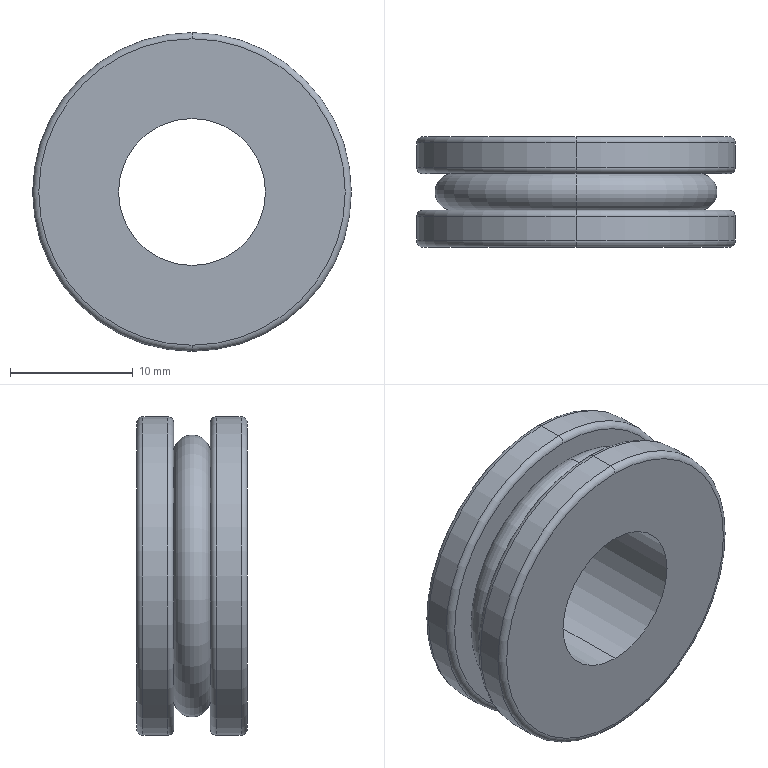Part | SolidWorks | features Fillet 1, Revolution 1 | 1 solid | 20 faces | box 26 x 9 x 26 mm | volume 3329 mm3 | torus 10 | cylinder 6 | plane 4 | commonest cylinder face diameters 26 x4 12 x2
STEP:
#1=CARTESIAN_POINT('',(0.,-3.,-12.5));
#2=VERTEX_POINT('',#1);
#3=CARTESIAN_POINT('',(0.,-3.,12.5));
#4=VERTEX_POINT('',#3);
#5=CARTESIAN_POINT('',(0.,-3.,0.));
#6=DIRECTION('',(0.,-1.,0.));
#7=DIRECTION('',(0.,0.,1.));
#8=AXIS2_PLACEMENT_3D('',#5,#6,#7);
#9=CIRCLE('',#8,12.5);
#10=EDGE_CURVE('',#2,#4,#9,.T.);
#11=ORIENTED_EDGE('',*,*,#10,.F.);
#12=CARTESIAN_POINT('',(0.,-2.5,-13.));
#13=VERTEX_POINT('',#12);
#14=CARTESIAN_POINT('',(0.,-2.5,-12.5));
#15=DIRECTION('',(1.,0.,0.));
#16=DIRECTION('',(0.,0.,-1.));
#17=AXIS2_PLACEMENT_3D('',#14,#15,#16);
#18=CIRCLE('',#17,0.5);
#19=EDGE_CURVE('',#2,#13,#18,.T.);
#20=ORIENTED_EDGE('',*,*,#19,.T.);
#21=CARTESIAN_POINT('',(0.,-2.5,13.));
#22=VERTEX_POINT('',#21);
#23=CARTESIAN_POINT('',(0.,-2.5,0.));
#24=DIRECTION('',(0.,1.,0.));
#25=DIRECTION('',(0.,0.,1.));
#26=AXIS2_PLACEMENT_3D('',#23,#24,#25);
#27=CIRCLE('',#26,13.);
#28=EDGE_CURVE('',#22,#13,#27,.T.);
#29=ORIENTED_EDGE('',*,*,#28,.F.);
#30=CARTESIAN_POINT('',(0.,-2.5,12.5));
#31=DIRECTION('',(-1.,0.,0.));
#32=DIRECTION('',(0.,0.,1.));
#33=AXIS2_PLACEMENT_3D('',#30,#31,#32);
#34=CIRCLE('',#33,0.5);
#35=EDGE_CURVE('',#4,#22,#34,.T.);
#36=ORIENTED_EDGE('',*,*,#35,.F.);
#37=EDGE_LOOP('',(#11,#20,#29,#36));
#38=FACE_OUTER_BOUND('',#37,.T.);
#39=CARTESIAN_POINT('',(0.,-2.5,0.));
#40=DIRECTION('',(0.,1.,0.));
#41=DIRECTION('',(0.,0.,1.));
#42=AXIS2_PLACEMENT_3D('',#39,#40,#41);
#43=TOROIDAL_SURFACE('',#42,12.5,0.5);
#44=ADVANCED_FACE('',(#38),#43,.T.);
#45=CARTESIAN_POINT('',(0.,0.,12.5));
#46=VERTEX_POINT('',#45);
#47=CARTESIAN_POINT('',(0.,0.,-12.5));
#48=VERTEX_POINT('',#47);
#49=CARTESIAN_POINT('',(0.,0.,0.));
#50=DIRECTION('',(0.,1.,0.));
#51=DIRECTION('',(0.,0.,-1.));
#52=AXIS2_PLACEMENT_3D('',#49,#50,#51);
#53=CIRCLE('',#52,12.5);
#54=EDGE_CURVE('',#46,#48,#53,.T.);
#55=ORIENTED_EDGE('',*,*,#54,.F.);
#56=CARTESIAN_POINT('',(0.,-0.5,13.));
#57=VERTEX_POINT('',#56);
#58=CARTESIAN_POINT('',(0.,-0.5,12.5));
#59=DIRECTION('',(1.,0.,0.));
#60=DIRECTION('',(0.,0.,-1.));
#61=AXIS2_PLACEMENT_3D('',#58,#59,#60);
#62=CIRCLE('',#61,0.5);
#63=EDGE_CURVE('',#46,#57,#62,.T.);
#64=ORIENTED_EDGE('',*,*,#63,.T.);
#65=CARTESIAN_POINT('',(0.,-0.5,-13.));
#66=VERTEX_POINT('',#65);
#67=CARTESIAN_POINT('',(0.,-0.5,0.));
#68=DIRECTION('',(0.,-1.,0.));
#69=DIRECTION('',(0.,0.,-1.));
#70=AXIS2_PLACEMENT_3D('',#67,#68,#69);
#71=CIRCLE('',#70,13.);
#72=EDGE_CURVE('',#66,#57,#71,.T.);
#73=ORIENTED_EDGE('',*,*,#72,.F.);
#74=CARTESIAN_POINT('',(0.,-0.5,-12.5));
#75=DIRECTION('',(-1.,0.,0.));
#76=DIRECTION('',(0.,0.,1.));
#77=AXIS2_PLACEMENT_3D('',#74,#75,#76);
#78=CIRCLE('',#77,0.5);
#79=EDGE_CURVE('',#48,#66,#78,.T.);
#80=ORIENTED_EDGE('',*,*,#79,.F.);
#81=EDGE_LOOP('',(#55,#64,#73,#80));
#82=FACE_OUTER_BOUND('',#81,.T.);
#83=CARTESIAN_POINT('',(0.,-0.5,0.));
#84=DIRECTION('',(0.,-1.,0.));
#85=DIRECTION('',(0.,0.,-1.));
#86=AXIS2_PLACEMENT_3D('',#83,#84,#85);
#87=TOROIDAL_SURFACE('',#86,12.5,0.5);
#88=ADVANCED_FACE('',(#82),#87,.T.);
#89=CARTESIAN_POINT('',(0.,-6.,12.5));
#90=VERTEX_POINT('',#89);
#91=CARTESIAN_POINT('',(0.,-6.,-12.5));
#92=VERTEX_POINT('',#91);
#93=CARTESIAN_POINT('',(0.,-6.,0.));
#94=DIRECTION('',(0.,1.,0.));
#95=DIRECTION('',(0.,0.,-1.));
#96=AXIS2_PLACEMENT_3D('',#93,#94,#95);
#97=CIRCLE('',#96,12.5);
#98=EDGE_CURVE('',#90,#92,#97,.T.);
#99=ORIENTED_EDGE('',*,*,#98,.F.);
#100=CARTESIAN_POINT('',(0.,-6.5,13.));
#101=VERTEX_POINT('',#100);
#102=CARTESIAN_POINT('',(0.,-6.5,12.5));
#103=DIRECTION('',(1.,0.,0.));
#104=DIRECTION('',(0.,0.,-1.));
#105=AXIS2_PLACEMENT_3D('',#102,#103,#104);
#106=CIRCLE('',#105,0.5);
#107=EDGE_CURVE('',#90,#101,#106,.T.);
#108=ORIENTED_EDGE('',*,*,#107,.T.);
#109=CARTESIAN_POINT('',(0.,-6.5,-13.));
#110=VERTEX_POINT('',#109);
#111=CARTESIAN_POINT('',(0.,-6.5,0.));
#112=DIRECTION('',(0.,-1.,0.));
#113=DIRECTION('',(0.,0.,-1.));
#114=AXIS2_PLACEMENT_3D('',#111,#112,#113);
#115=CIRCLE('',#114,13.);
#116=EDGE_CURVE('',#110,#101,#115,.T.);
#117=ORIENTED_EDGE('',*,*,#116,.F.);
#118=CARTESIAN_POINT('',(0.,-6.5,-12.5));
#119=DIRECTION('',(-1.,0.,0.));
#120=DIRECTION('',(0.,0.,1.));
#121=AXIS2_PLACEMENT_3D('',#118,#119,#120);
#122=CIRCLE('',#121,0.5);
#123=EDGE_CURVE('',#92,#110,#122,.T.);
#124=ORIENTED_EDGE('',*,*,#123,.F.);
#125=EDGE_LOOP('',(#99,#108,#117,#124));
#126=FACE_OUTER_BOUND('',#125,.T.);
#127=CARTESIAN_POINT('',(0.,-6.5,0.));
#128=DIRECTION('',(0.,-1.,0.));
#129=DIRECTION('',(0.,0.,-1.));
#130=AXIS2_PLACEMENT_3D('',#127,#128,#129);
#131=TOROIDAL_SURFACE('',#130,12.5,0.5);
#132=ADVANCED_FACE('',(#126),#131,.T.);
#133=CARTESIAN_POINT('',(0.,-9.,-12.5));
#134=VERTEX_POINT('',#133);
#135=CARTESIAN_POINT('',(0.,-9.,12.5));
#136=VERTEX_POINT('',#135);
#137=CARTESIAN_POINT('',(0.,-9.,0.));
#138=DIRECTION('',(0.,-1.,0.));
#139=DIRECTION('',(0.,0.,1.));
#140=AXIS2_PLACEMENT_3D('',#137,#138,#139);
#141=CIRCLE('',#140,12.5);
#142=EDGE_CURVE('',#134,#136,#141,.T.);
#143=ORIENTED_EDGE('',*,*,#142,.F.);
#144=CARTESIAN_POINT('',(0.,-8.5,-13.));
#145=VERTEX_POINT('',#144);
#146=CARTESIAN_POINT('',(0.,-8.5,-12.5));
#147=DIRECTION('',(1.,0.,0.));
#148=DIRECTION('',(0.,0.,-1.));
#149=AXIS2_PLACEMENT_3D('',#146,#147,#148);
#150=CIRCLE('',#149,0.5);
#151=EDGE_CURVE('',#134,#145,#150,.T.);
#152=ORIENTED_EDGE('',*,*,#151,.T.);
#153=CARTESIAN_POINT('',(0.,-8.5,13.));
#154=VERTEX_POINT('',#153);
#155=CARTESIAN_POINT('',(0.,-8.5,0.));
#156=DIRECTION('',(0.,1.,0.));
#157=DIRECTION('',(0.,0.,1.));
#158=AXIS2_PLACEMENT_3D('',#155,#156,#157);
#159=CIRCLE('',#158,13.);
#160=EDGE_CURVE('',#154,#145,#159,.T.);
#161=ORIENTED_EDGE('',*,*,#160,.F.);
#162=CARTESIAN_POINT('',(0.,-8.5,12.5));
#163=DIRECTION('',(-1.,0.,0.));
#164=DIRECTION('',(0.,0.,1.));
#165=AXIS2_PLACEMENT_3D('',#162,#163,#164);
#166=CIRCLE('',#165,0.5);
#167=EDGE_CURVE('',#136,#154,#166,.T.);
#168=ORIENTED_EDGE('',*,*,#167,.F.);
#169=EDGE_LOOP('',(#143,#152,#161,#168));
#170=FACE_OUTER_BOUND('',#169,.T.);
#171=CARTESIAN_POINT('',(0.,-8.5,0.));
#172=DIRECTION('',(0.,1.,0.));
#173=DIRECTION('',(0.,0.,1.));
#174=AXIS2_PLACEMENT_3D('',#171,#172,#173);
#175=TOROIDAL_SURFACE('',#174,12.5,0.5);
#176=ADVANCED_FACE('',(#170),#175,.T.);
#177=CARTESIAN_POINT('',(0.,-9.,-6.));
#178=VERTEX_POINT('',#177);
#179=CARTESIAN_POINT('',(0.,-9.,6.));
#180=VERTEX_POINT('',#179);
#181=CARTESIAN_POINT('',(0.,-9.,0.));
#182=DIRECTION('',(0.,1.,0.));
#183=DIRECTION('',(0.,0.,1.));
#184=AXIS2_PLACEMENT_3D('',#181,#182,#183);
#185=CIRCLE('',#184,6.);
#186=EDGE_CURVE('',#178,#180,#185,.T.);
#187=ORIENTED_EDGE('',*,*,#186,.F.);
#188=CARTESIAN_POINT('',(0.,0.,-6.));
#189=VERTEX_POINT('',#188);
#190=CARTESIAN_POINT('',(0.,0.,-6.));
#191=DIRECTION('',(0.,1.,0.));
#192=VECTOR('',#191,1000.);
#193=LINE('',#190,#192);
#194=EDGE_CURVE('',#178,#189,#193,.T.);
#195=ORIENTED_EDGE('',*,*,#194,.T.);
#196=CARTESIAN_POINT('',(0.,0.,6.));
#197=VERTEX_POINT('',#196);
#198=CARTESIAN_POINT('',(0.,0.,0.));
#199=DIRECTION('',(0.,1.,0.));
#200=DIRECTION('',(0.,0.,1.));
#201=AXIS2_PLACEMENT_3D('',#198,#199,#200);
#202=CIRCLE('',#201,6.);
#203=EDGE_CURVE('',#189,#197,#202,.T.);
#204=ORIENTED_EDGE('',*,*,#203,.T.);
#205=CARTESIAN_POINT('',(0.,0.,6.));
#206=DIRECTION('',(0.,1.,0.));
#207=VECTOR('',#206,1000.);
#208=LINE('',#205,#207);
#209=EDGE_CURVE('',#180,#197,#208,.T.);
#210=ORIENTED_EDGE('',*,*,#209,.F.);
#211=EDGE_LOOP('',(#187,#195,#204,#210));
#212=FACE_OUTER_BOUND('',#211,.T.);
#213=CARTESIAN_POINT('',(0.,0.,0.));
#214=DIRECTION('',(0.,1.,0.));
#215=DIRECTION('',(0.,0.,1.));
#216=AXIS2_PLACEMENT_3D('',#213,#214,#215);
#217=CYLINDRICAL_SURFACE('',#216,6.);
#218=ADVANCED_FACE('',(#212),#217,.F.);
#219=ORIENTED_EDGE('',*,*,#160,.T.);
#220=CARTESIAN_POINT('',(0.,0.,-13.));
#221=DIRECTION('',(0.,1.,0.));
#222=VECTOR('',#221,1000.);
#223=LINE('',#220,#222);
#224=EDGE_CURVE('',#145,#110,#223,.T.);
#225=ORIENTED_EDGE('',*,*,#224,.T.);
#226=ORIENTED_EDGE('',*,*,#116,.T.);
#227=CARTESIAN_POINT('',(0.,0.,13.));
#228=DIRECTION('',(0.,1.,0.));
#229=VECTOR('',#228,1000.);
#230=LINE('',#227,#229);
#231=EDGE_CURVE('',#154,#101,#230,.T.);
#232=ORIENTED_EDGE('',*,*,#231,.F.);
#233=EDGE_LOOP('',(#219,#225,#226,#232));
#234=FACE_OUTER_BOUND('',#233,.T.);
#235=CARTESIAN_POINT('',(0.,0.,0.));
#236=DIRECTION('',(0.,1.,0.));
#237=DIRECTION('',(0.,0.,1.));
#238=AXIS2_PLACEMENT_3D('',#235,#236,#237);
#239=CYLINDRICAL_SURFACE('',#238,13.);
#240=ADVANCED_FACE('',(#234),#239,.T.);
#241=CARTESIAN_POINT('',(0.,-6.,10.));
#242=VERTEX_POINT('',#241);
#243=CARTESIAN_POINT('',(0.,-6.,-10.));
#244=VERTEX_POINT('',#243);
#245=CARTESIAN_POINT('',(0.,-6.,0.));
#246=DIRECTION('',(0.,1.,0.));
#247=DIRECTION('',(0.,0.,1.));
#248=AXIS2_PLACEMENT_3D('',#245,#246,#247);
#249=CIRCLE('',#248,10.);
#250=EDGE_CURVE('',#242,#244,#249,.T.);
#251=ORIENTED_EDGE('',*,*,#250,.T.);
#252=CARTESIAN_POINT('',(0.,-3.,-10.));
#253=VERTEX_POINT('',#252);
#254=CARTESIAN_POINT('',(0.,-4.5,-10.));
#255=DIRECTION('',(1.,0.,0.));
#256=DIRECTION('',(0.,0.,-1.));
#257=AXIS2_PLACEMENT_3D('',#254,#255,#256);
#258=CIRCLE('',#257,1.5);
#259=EDGE_CURVE('',#244,#253,#258,.T.);
#260=ORIENTED_EDGE('',*,*,#259,.T.);
#261=CARTESIAN_POINT('',(0.,-3.,10.));
#262=VERTEX_POINT('',#261);
#263=CARTESIAN_POINT('',(0.,-3.,0.));
#264=DIRECTION('',(0.,1.,0.));
#265=DIRECTION('',(0.,0.,1.));
#266=AXIS2_PLACEMENT_3D('',#263,#264,#265);
#267=CIRCLE('',#266,10.);
#268=EDGE_CURVE('',#262,#253,#267,.T.);
#269=ORIENTED_EDGE('',*,*,#268,.F.);
#270=CARTESIAN_POINT('',(0.,-4.5,10.));
#271=DIRECTION('',(-1.,0.,0.));
#272=DIRECTION('',(0.,0.,1.));
#273=AXIS2_PLACEMENT_3D('',#270,#271,#272);
#274=CIRCLE('',#273,1.5);
#275=EDGE_CURVE('',#242,#262,#274,.T.);
#276=ORIENTED_EDGE('',*,*,#275,.F.);
#277=EDGE_LOOP('',(#251,#260,#269,#276));
#278=FACE_OUTER_BOUND('',#277,.T.);
#279=CARTESIAN_POINT('',(0.,-4.5,0.));
#280=DIRECTION('',(0.,1.,0.));
#281=DIRECTION('',(0.,0.,1.));
#282=AXIS2_PLACEMENT_3D('',#279,#280,#281);
#283=TOROIDAL_SURFACE('',#282,10.,1.5);
#284=ADVANCED_FACE('',(#278),#283,.T.);
#285=ORIENTED_EDGE('',*,*,#28,.T.);
#286=CARTESIAN_POINT('',(0.,0.,-13.));
#287=DIRECTION('',(0.,1.,0.));
#288=VECTOR('',#287,1000.);
#289=LINE('',#286,#288);
#290=EDGE_CURVE('',#13,#66,#289,.T.);
#291=ORIENTED_EDGE('',*,*,#290,.T.);
#292=ORIENTED_EDGE('',*,*,#72,.T.);
#293=CARTESIAN_POINT('',(0.,0.,13.));
#294=DIRECTION('',(0.,1.,0.));
#295=VECTOR('',#294,1000.);
#296=LINE('',#293,#295);
#297=EDGE_CURVE('',#22,#57,#296,.T.);
#298=ORIENTED_EDGE('',*,*,#297,.F.);
#299=EDGE_LOOP('',(#285,#291,#292,#298));
#300=FACE_OUTER_BOUND('',#299,.T.);
#301=CARTESIAN_POINT('',(0.,0.,0.));
#302=DIRECTION('',(0.,1.,0.));
#303=DIRECTION('',(0.,0.,1.));
#304=AXIS2_PLACEMENT_3D('',#301,#302,#303);
#305=CYLINDRICAL_SURFACE('',#304,13.);
#306=ADVANCED_FACE('',(#300),#305,.T.);
#307=ORIENTED_EDGE('',*,*,#290,.F.);
#308=CARTESIAN_POINT('',(0.,-2.5,0.));
#309=DIRECTION('',(0.,1.,0.));
#310=DIRECTION('',(0.,0.,1.));
#311=AXIS2_PLACEMENT_3D('',#308,#309,#310);
#312=CIRCLE('',#311,13.);
#313=EDGE_CURVE('',#13,#22,#312,.T.);
#314=ORIENTED_EDGE('',*,*,#313,.T.);
#315=ORIENTED_EDGE('',*,*,#297,.T.);
#316=CARTESIAN_POINT('',(0.,-0.5,0.));
#317=DIRECTION('',(0.,-1.,0.));
#318=DIRECTION('',(0.,0.,-1.));
#319=AXIS2_PLACEMENT_3D('',#316,#317,#318);
#320=CIRCLE('',#319,13.);
#321=EDGE_CURVE('',#57,#66,#320,.T.);
#322=ORIENTED_EDGE('',*,*,#321,.T.);
#323=EDGE_LOOP('',(#307,#314,#315,#322));
#324=FACE_OUTER_BOUND('',#323,.T.);
#325=CARTESIAN_POINT('',(0.,0.,0.));
#326=DIRECTION('',(0.,1.,0.));
#327=DIRECTION('',(0.,0.,1.));
#328=AXIS2_PLACEMENT_3D('',#325,#326,#327);
#329=CYLINDRICAL_SURFACE('',#328,13.);
#330=ADVANCED_FACE('',(#324),#329,.T.);
#331=CARTESIAN_POINT('',(0.,-3.,0.));
#332=DIRECTION('',(0.,-1.,0.));
#333=DIRECTION('',(0.,0.,1.));
#334=AXIS2_PLACEMENT_3D('',#331,#332,#333);
#335=CIRCLE('',#334,12.5);
#336=EDGE_CURVE('',#4,#2,#335,.T.);
#337=ORIENTED_EDGE('',*,*,#336,.T.);
#338=ORIENTED_EDGE('',*,*,#10,.T.);
#339=EDGE_LOOP('',(#337,#338));
#340=FACE_OUTER_BOUND('',#339,.T.);
#341=ORIENTED_EDGE('',*,*,#268,.T.);
#342=CARTESIAN_POINT('',(0.,-3.,0.));
#343=DIRECTION('',(0.,1.,0.));
#344=DIRECTION('',(0.,0.,1.));
#345=AXIS2_PLACEMENT_3D('',#342,#343,#344);
#346=CIRCLE('',#345,10.);
#347=EDGE_CURVE('',#253,#262,#346,.T.);
#348=ORIENTED_EDGE('',*,*,#347,.T.);
#349=EDGE_LOOP('',(#341,#348));
#350=FACE_BOUND('',#349,.T.);
#351=CARTESIAN_POINT('',(13.,-3.,0.));
#352=DIRECTION('',(0.,1.,0.));
#353=DIRECTION('',(0.,0.,1.));
#354=AXIS2_PLACEMENT_3D('',#351,#352,#353);
#355=PLANE('',#354);
#356=ADVANCED_FACE('',(#340,#350),#355,.F.);
#357=ORIENTED_EDGE('',*,*,#259,.F.);
#358=CARTESIAN_POINT('',(0.,-6.,0.));
#359=DIRECTION('',(0.,1.,0.));
#360=DIRECTION('',(0.,0.,1.));
#361=AXIS2_PLACEMENT_3D('',#358,#359,#360);
#362=CIRCLE('',#361,10.);
#363=EDGE_CURVE('',#244,#242,#362,.T.);
#364=ORIENTED_EDGE('',*,*,#363,.T.);
#365=ORIENTED_EDGE('',*,*,#275,.T.);
#366=ORIENTED_EDGE('',*,*,#347,.F.);
#367=EDGE_LOOP('',(#357,#364,#365,#366));
#368=FACE_OUTER_BOUND('',#367,.T.);
#369=CARTESIAN_POINT('',(0.,-4.5,0.));
#370=DIRECTION('',(0.,1.,0.));
#371=DIRECTION('',(0.,0.,1.));
#372=AXIS2_PLACEMENT_3D('',#369,#370,#371);
#373=TOROIDAL_SURFACE('',#372,10.,1.5);
#374=ADVANCED_FACE('',(#368),#373,.T.);
#375=CARTESIAN_POINT('',(0.,-6.,0.));
#376=DIRECTION('',(0.,1.,0.));
#377=DIRECTION('',(0.,0.,-1.));
#378=AXIS2_PLACEMENT_3D('',#375,#376,#377);
#379=CIRCLE('',#378,12.5);
#380=EDGE_CURVE('',#92,#90,#379,.T.);
#381=ORIENTED_EDGE('',*,*,#380,.T.);
#382=ORIENTED_EDGE('',*,*,#98,.T.);
#383=EDGE_LOOP('',(#381,#382));
#384=FACE_OUTER_BOUND('',#383,.T.);
#385=ORIENTED_EDGE('',*,*,#250,.F.);
#386=ORIENTED_EDGE('',*,*,#363,.F.);
#387=EDGE_LOOP('',(#385,#386));
#388=FACE_BOUND('',#387,.T.);
#389=CARTESIAN_POINT('',(10.,-6.,0.));
#390=DIRECTION('',(0.,-1.,0.));
#391=DIRECTION('',(0.,0.,-1.));
#392=AXIS2_PLACEMENT_3D('',#389,#390,#391);
#393=PLANE('',#392);
#394=ADVANCED_FACE('',(#384,#388),#393,.F.);
#395=ORIENTED_EDGE('',*,*,#224,.F.);
#396=CARTESIAN_POINT('',(0.,-8.5,0.));
#397=DIRECTION('',(0.,1.,0.));
#398=DIRECTION('',(0.,0.,1.));
#399=AXIS2_PLACEMENT_3D('',#396,#397,#398);
#400=CIRCLE('',#399,13.);
#401=EDGE_CURVE('',#145,#154,#400,.T.);
#402=ORIENTED_EDGE('',*,*,#401,.T.);
#403=ORIENTED_EDGE('',*,*,#231,.T.);
#404=CARTESIAN_POINT('',(0.,-6.5,0.));
#405=DIRECTION('',(0.,-1.,0.));
#406=DIRECTION('',(0.,0.,-1.));
#407=AXIS2_PLACEMENT_3D('',#404,#405,#406);
#408=CIRCLE('',#407,13.);
#409=EDGE_CURVE('',#101,#110,#408,.T.);
#410=ORIENTED_EDGE('',*,*,#409,.T.);
#411=EDGE_LOOP('',(#395,#402,#403,#410));
#412=FACE_OUTER_BOUND('',#411,.T.);
#413=CARTESIAN_POINT('',(0.,0.,0.));
#414=DIRECTION('',(0.,1.,0.));
#415=DIRECTION('',(0.,0.,1.));
#416=AXIS2_PLACEMENT_3D('',#413,#414,#415);
#417=CYLINDRICAL_SURFACE('',#416,13.);
#418=ADVANCED_FACE('',(#412),#417,.T.);
#419=CARTESIAN_POINT('',(0.,-9.,0.));
#420=DIRECTION('',(0.,-1.,0.));
#421=DIRECTION('',(0.,0.,1.));
#422=AXIS2_PLACEMENT_3D('',#419,#420,#421);
#423=CIRCLE('',#422,12.5);
#424=EDGE_CURVE('',#136,#134,#423,.T.);
#425=ORIENTED_EDGE('',*,*,#424,.T.);
#426=ORIENTED_EDGE('',*,*,#142,.T.);
#427=EDGE_LOOP('',(#425,#426));
#428=FACE_OUTER_BOUND('',#427,.T.);
#429=CARTESIAN_POINT('',(0.,-9.,0.));
#430=DIRECTION('',(0.,1.,0.));
#431=DIRECTION('',(0.,0.,1.));
#432=AXIS2_PLACEMENT_3D('',#429,#430,#431);
#433=CIRCLE('',#432,6.);
#434=EDGE_CURVE('',#180,#178,#433,.T.);
#435=ORIENTED_EDGE('',*,*,#434,.T.);
#436=ORIENTED_EDGE('',*,*,#186,.T.);
#437=EDGE_LOOP('',(#435,#436));
#438=FACE_BOUND('',#437,.T.);
#439=CARTESIAN_POINT('',(13.,-9.,0.));
#440=DIRECTION('',(0.,1.,0.));
#441=DIRECTION('',(0.,0.,1.));
#442=AXIS2_PLACEMENT_3D('',#439,#440,#441);
#443=PLANE('',#442);
#444=ADVANCED_FACE('',(#428,#438),#443,.F.);
#445=ORIENTED_EDGE('',*,*,#194,.F.);
#446=ORIENTED_EDGE('',*,*,#434,.F.);
#447=ORIENTED_EDGE('',*,*,#209,.T.);
#448=CARTESIAN_POINT('',(0.,0.,0.));
#449=DIRECTION('',(0.,1.,0.));
#450=DIRECTION('',(0.,0.,1.));
#451=AXIS2_PLACEMENT_3D('',#448,#449,#450);
#452=CIRCLE('',#451,6.);
#453=EDGE_CURVE('',#197,#189,#452,.T.);
#454=ORIENTED_EDGE('',*,*,#453,.T.);
#455=EDGE_LOOP('',(#445,#446,#447,#454));
#456=FACE_OUTER_BOUND('',#455,.T.);
#457=CARTESIAN_POINT('',(0.,0.,0.));
#458=DIRECTION('',(0.,1.,0.));
#459=DIRECTION('',(0.,0.,1.));
#460=AXIS2_PLACEMENT_3D('',#457,#458,#459);
#461=CYLINDRICAL_SURFACE('',#460,6.);
#462=ADVANCED_FACE('',(#456),#461,.F.);
#463=CARTESIAN_POINT('',(0.,0.,0.));
#464=DIRECTION('',(0.,1.,0.));
#465=DIRECTION('',(0.,0.,-1.));
#466=AXIS2_PLACEMENT_3D('',#463,#464,#465);
#467=CIRCLE('',#466,12.5);
#468=EDGE_CURVE('',#48,#46,#467,.T.);
#469=ORIENTED_EDGE('',*,*,#468,.T.);
#470=ORIENTED_EDGE('',*,*,#54,.T.);
#471=EDGE_LOOP('',(#469,#470));
#472=FACE_OUTER_BOUND('',#471,.T.);
#473=ORIENTED_EDGE('',*,*,#453,.F.);
#474=ORIENTED_EDGE('',*,*,#203,.F.);
#475=EDGE_LOOP('',(#473,#474));
#476=FACE_BOUND('',#475,.T.);
#477=CARTESIAN_POINT('',(6.,0.,0.));
#478=DIRECTION('',(0.,-1.,0.));
#479=DIRECTION('',(0.,0.,-1.));
#480=AXIS2_PLACEMENT_3D('',#477,#478,#479);
#481=PLANE('',#480);
#482=ADVANCED_FACE('',(#472,#476),#481,.F.);
#483=ORIENTED_EDGE('',*,*,#151,.F.);
#484=ORIENTED_EDGE('',*,*,#424,.F.);
#485=ORIENTED_EDGE('',*,*,#167,.T.);
#486=ORIENTED_EDGE('',*,*,#401,.F.);
#487=EDGE_LOOP('',(#483,#484,#485,#486));
#488=FACE_OUTER_BOUND('',#487,.T.);
#489=CARTESIAN_POINT('',(0.,-8.5,0.));
#490=DIRECTION('',(0.,1.,0.));
#491=DIRECTION('',(0.,0.,1.));
#492=AXIS2_PLACEMENT_3D('',#489,#490,#491);
#493=TOROIDAL_SURFACE('',#492,12.5,0.5);
#494=ADVANCED_FACE('',(#488),#493,.T.);
#495=ORIENTED_EDGE('',*,*,#107,.F.);
#496=ORIENTED_EDGE('',*,*,#380,.F.);
#497=ORIENTED_EDGE('',*,*,#123,.T.);
#498=ORIENTED_EDGE('',*,*,#409,.F.);
#499=EDGE_LOOP('',(#495,#496,#497,#498));
#500=FACE_OUTER_BOUND('',#499,.T.);
#501=CARTESIAN_POINT('',(0.,-6.5,0.));
#502=DIRECTION('',(0.,-1.,0.));
#503=DIRECTION('',(0.,0.,-1.));
#504=AXIS2_PLACEMENT_3D('',#501,#502,#503);
#505=TOROIDAL_SURFACE('',#504,12.5,0.5);
#506=ADVANCED_FACE('',(#500),#505,.T.);
#507=ORIENTED_EDGE('',*,*,#63,.F.);
#508=ORIENTED_EDGE('',*,*,#468,.F.);
#509=ORIENTED_EDGE('',*,*,#79,.T.);
#510=ORIENTED_EDGE('',*,*,#321,.F.);
#511=EDGE_LOOP('',(#507,#508,#509,#510));
#512=FACE_OUTER_BOUND('',#511,.T.);
#513=CARTESIAN_POINT('',(0.,-0.5,0.));
#514=DIRECTION('',(0.,-1.,0.));
#515=DIRECTION('',(0.,0.,-1.));
#516=AXIS2_PLACEMENT_3D('',#513,#514,#515);
#517=TOROIDAL_SURFACE('',#516,12.5,0.5);
#518=ADVANCED_FACE('',(#512),#517,.T.);
#519=ORIENTED_EDGE('',*,*,#19,.F.);
#520=ORIENTED_EDGE('',*,*,#336,.F.);
#521=ORIENTED_EDGE('',*,*,#35,.T.);
#522=ORIENTED_EDGE('',*,*,#313,.F.);
#523=EDGE_LOOP('',(#519,#520,#521,#522));
#524=FACE_OUTER_BOUND('',#523,.T.);
#525=CARTESIAN_POINT('',(0.,-2.5,0.));
#526=DIRECTION('',(0.,1.,0.));
#527=DIRECTION('',(0.,0.,1.));
#528=AXIS2_PLACEMENT_3D('',#525,#526,#527);
#529=TOROIDAL_SURFACE('',#528,12.5,0.5);
#530=ADVANCED_FACE('',(#524),#529,.T.);
#531=CLOSED_SHELL('',(#44,#88,#132,#176,#218,#240,#284,#306,#330,#356,#374,#394,#418,#444,#462,#482,#494,#506,#518,#530));
#532=MANIFOLD_SOLID_BREP('',#531);
#533=CARTESIAN_POINT('',(0.,0.,0.));
#534=DIRECTION('',(0.,0.,1.));
#535=DIRECTION('',(1.,0.,0.));
#536=AXIS2_PLACEMENT_3D('',#533,#534,#535);
#537=(LENGTH_UNIT()NAMED_UNIT(*)SI_UNIT(.MILLI.,.METRE.));
#538=UNCERTAINTY_MEASURE_WITH_UNIT(LENGTH_MEASURE(0.00001),#537,'','');
#539=(NAMED_UNIT(*)PLANE_ANGLE_UNIT()SI_UNIT($,.RADIAN.));
#540=(NAMED_UNIT(*)SI_UNIT($,.STERADIAN.)SOLID_ANGLE_UNIT());
#541=(GEOMETRIC_REPRESENTATION_CONTEXT(3)GLOBAL_UNCERTAINTY_ASSIGNED_CONTEXT((#538))GLOBAL_UNIT_ASSIGNED_CONTEXT((#537,#539,#540))REPRESENTATION_CONTEXT('',''));
#542=ADVANCED_BREP_SHAPE_REPRESENTATION('',(#532,#536),#541);